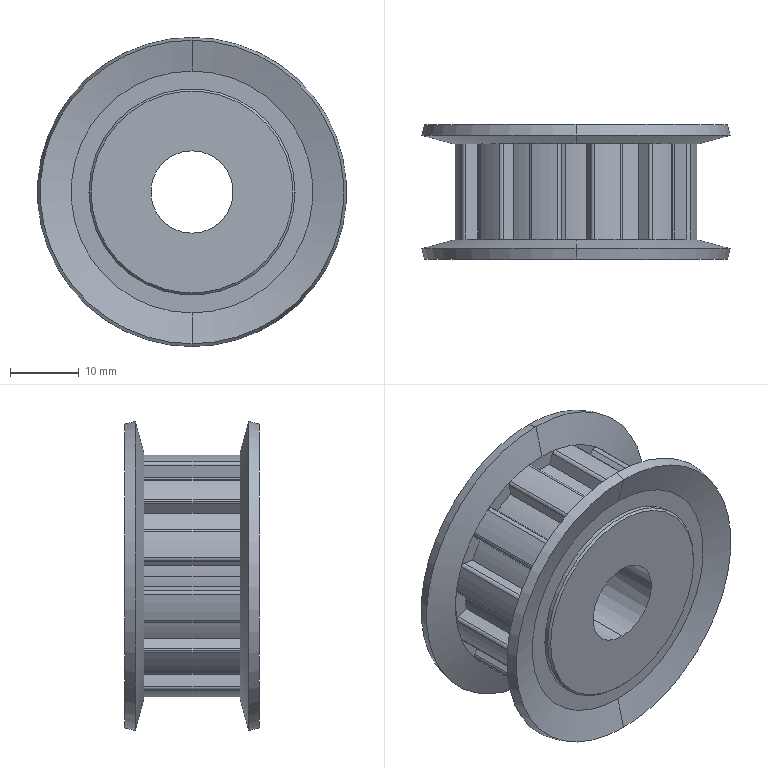Part | STEP file | 0243_Z_ATPP12L050-A-P12-KC90_2 | 1 solid | 137 faces | box 45 x 19.604 x 45 mm | volume 16570 mm3 | cylinder 69 | plane 52 | cone 16 | commonest cylinder face diameters 1.06 x30 31.36 x15 35.62 x12 3.3 x4 30 x4 1.72 x2